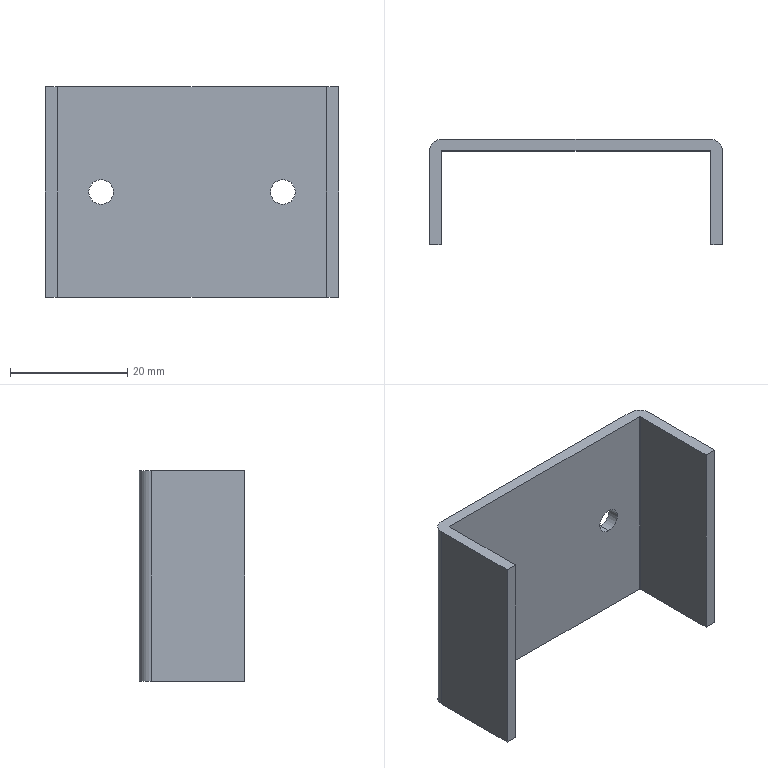Part | STEP file | Closing Plate Clip | 1 solid | 18 faces | box 50 x 18 x 36 mm | volume 5781 mm3 | plane 10 | cylinder 8 | commonest cylinder face diameters 4.2 x6 0.2 x2
STEP:
#1=CARTESIAN_POINT('',(-37.108,9.693,15.9));
#2=VERTEX_POINT('',#1);
#3=CARTESIAN_POINT('',(-37.108,9.693,20.1));
#4=VERTEX_POINT('',#3);
#5=CARTESIAN_POINT('',(-37.108,9.693,18.));
#6=DIRECTION('',(0.,1.,0.));
#7=DIRECTION('',(0.,0.,1.));
#8=AXIS2_PLACEMENT_3D('',#5,#6,#7);
#9=CIRCLE('',#8,2.1);
#10=EDGE_CURVE('',#2,#4,#9,.T.);
#11=ORIENTED_EDGE('',*,*,#10,.F.);
#12=CARTESIAN_POINT('',(-37.108,11.693,15.9));
#13=VERTEX_POINT('',#12);
#14=CARTESIAN_POINT('',(-37.108,1.693,15.9));
#15=DIRECTION('',(0.,1.,0.));
#16=VECTOR('',#15,1000.);
#17=LINE('',#14,#16);
#18=EDGE_CURVE('',#2,#13,#17,.T.);
#19=ORIENTED_EDGE('',*,*,#18,.T.);
#20=CARTESIAN_POINT('',(-37.108,11.693,20.1));
#21=VERTEX_POINT('',#20);
#22=CARTESIAN_POINT('',(-37.108,11.693,18.));
#23=DIRECTION('',(0.,-1.,0.));
#24=DIRECTION('',(0.,0.,1.));
#25=AXIS2_PLACEMENT_3D('',#22,#23,#24);
#26=CIRCLE('',#25,2.1);
#27=EDGE_CURVE('',#21,#13,#26,.T.);
#28=ORIENTED_EDGE('',*,*,#27,.F.);
#29=CARTESIAN_POINT('',(-37.108,1.693,20.1));
#30=DIRECTION('',(0.,1.,0.));
#31=VECTOR('',#30,1000.);
#32=LINE('',#29,#31);
#33=EDGE_CURVE('',#4,#21,#32,.T.);
#34=ORIENTED_EDGE('',*,*,#33,.F.);
#35=EDGE_LOOP('',(#11,#19,#28,#34));
#36=FACE_OUTER_BOUND('',#35,.T.);
#37=CARTESIAN_POINT('',(-37.108,1.693,18.));
#38=DIRECTION('',(0.,1.,0.));
#39=DIRECTION('',(0.,0.,1.));
#40=AXIS2_PLACEMENT_3D('',#37,#38,#39);
#41=CYLINDRICAL_SURFACE('',#40,2.1);
#42=ADVANCED_FACE('',(#36),#41,.F.);
#43=CARTESIAN_POINT('',(-6.108,9.693,15.9));
#44=VERTEX_POINT('',#43);
#45=CARTESIAN_POINT('',(-6.108,9.693,20.1));
#46=VERTEX_POINT('',#45);
#47=CARTESIAN_POINT('',(-6.108,9.693,18.));
#48=DIRECTION('',(0.,1.,0.));
#49=DIRECTION('',(0.,0.,1.));
#50=AXIS2_PLACEMENT_3D('',#47,#48,#49);
#51=CIRCLE('',#50,2.1);
#52=EDGE_CURVE('',#44,#46,#51,.T.);
#53=ORIENTED_EDGE('',*,*,#52,.F.);
#54=CARTESIAN_POINT('',(-6.108,11.693,15.9));
#55=VERTEX_POINT('',#54);
#56=CARTESIAN_POINT('',(-6.108,1.693,15.9));
#57=DIRECTION('',(0.,1.,0.));
#58=VECTOR('',#57,1000.);
#59=LINE('',#56,#58);
#60=EDGE_CURVE('',#44,#55,#59,.T.);
#61=ORIENTED_EDGE('',*,*,#60,.T.);
#62=CARTESIAN_POINT('',(-6.108,11.693,20.1));
#63=VERTEX_POINT('',#62);
#64=CARTESIAN_POINT('',(-6.108,11.693,18.));
#65=DIRECTION('',(0.,-1.,0.));
#66=DIRECTION('',(0.,0.,1.));
#67=AXIS2_PLACEMENT_3D('',#64,#65,#66);
#68=CIRCLE('',#67,2.1);
#69=EDGE_CURVE('',#63,#55,#68,.T.);
#70=ORIENTED_EDGE('',*,*,#69,.F.);
#71=CARTESIAN_POINT('',(-6.108,1.693,20.1));
#72=DIRECTION('',(0.,1.,0.));
#73=VECTOR('',#72,1000.);
#74=LINE('',#71,#73);
#75=EDGE_CURVE('',#46,#63,#74,.T.);
#76=ORIENTED_EDGE('',*,*,#75,.F.);
#77=EDGE_LOOP('',(#53,#61,#70,#76));
#78=FACE_OUTER_BOUND('',#77,.T.);
#79=CARTESIAN_POINT('',(-6.108,1.693,18.));
#80=DIRECTION('',(0.,1.,0.));
#81=DIRECTION('',(0.,0.,1.));
#82=AXIS2_PLACEMENT_3D('',#79,#80,#81);
#83=CYLINDRICAL_SURFACE('',#82,2.1);
#84=ADVANCED_FACE('',(#78),#83,.F.);
#85=CARTESIAN_POINT('',(-44.508,11.693,36.));
#86=VERTEX_POINT('',#85);
#87=CARTESIAN_POINT('',(1.292,11.693,36.));
#88=VERTEX_POINT('',#87);
#89=CARTESIAN_POINT('',(-46.608,11.693,36.));
#90=DIRECTION('',(1.,0.,0.));
#91=VECTOR('',#90,1000.);
#92=LINE('',#89,#91);
#93=EDGE_CURVE('',#86,#88,#92,.T.);
#94=ORIENTED_EDGE('',*,*,#93,.T.);
#95=CARTESIAN_POINT('',(1.292,11.693,0.));
#96=VERTEX_POINT('',#95);
#97=CARTESIAN_POINT('',(1.292,11.693,36.));
#98=DIRECTION('',(0.,0.,-1.));
#99=VECTOR('',#98,1000.);
#100=LINE('',#97,#99);
#101=EDGE_CURVE('',#88,#96,#100,.T.);
#102=ORIENTED_EDGE('',*,*,#101,.T.);
#103=CARTESIAN_POINT('',(-44.508,11.693,0.));
#104=VERTEX_POINT('',#103);
#105=CARTESIAN_POINT('',(-46.608,11.693,0.));
#106=DIRECTION('',(-1.,0.,0.));
#107=VECTOR('',#106,1000.);
#108=LINE('',#105,#107);
#109=EDGE_CURVE('',#96,#104,#108,.T.);
#110=ORIENTED_EDGE('',*,*,#109,.T.);
#111=CARTESIAN_POINT('',(-44.508,11.693,36.));
#112=DIRECTION('',(0.,0.,1.));
#113=VECTOR('',#112,1000.);
#114=LINE('',#111,#113);
#115=EDGE_CURVE('',#104,#86,#114,.T.);
#116=ORIENTED_EDGE('',*,*,#115,.T.);
#117=EDGE_LOOP('',(#94,#102,#110,#116));
#118=FACE_OUTER_BOUND('',#117,.T.);
#119=ORIENTED_EDGE('',*,*,#27,.T.);
#120=CARTESIAN_POINT('',(-37.108,11.693,18.));
#121=DIRECTION('',(0.,-1.,0.));
#122=DIRECTION('',(0.,0.,1.));
#123=AXIS2_PLACEMENT_3D('',#120,#121,#122);
#124=CIRCLE('',#123,2.1);
#125=EDGE_CURVE('',#13,#21,#124,.T.);
#126=ORIENTED_EDGE('',*,*,#125,.T.);
#127=EDGE_LOOP('',(#119,#126));
#128=FACE_BOUND('',#127,.T.);
#129=ORIENTED_EDGE('',*,*,#69,.T.);
#130=CARTESIAN_POINT('',(-6.108,11.693,18.));
#131=DIRECTION('',(0.,-1.,0.));
#132=DIRECTION('',(0.,0.,1.));
#133=AXIS2_PLACEMENT_3D('',#130,#131,#132);
#134=CIRCLE('',#133,2.1);
#135=EDGE_CURVE('',#55,#63,#134,.T.);
#136=ORIENTED_EDGE('',*,*,#135,.T.);
#137=EDGE_LOOP('',(#129,#136));
#138=FACE_BOUND('',#137,.T.);
#139=CARTESIAN_POINT('',(-46.608,11.693,36.));
#140=DIRECTION('',(0.,1.,0.));
#141=DIRECTION('',(0.,0.,1.));
#142=AXIS2_PLACEMENT_3D('',#139,#140,#141);
#143=PLANE('',#142);
#144=ADVANCED_FACE('',(#118,#128,#138),#143,.T.);
#145=CARTESIAN_POINT('',(3.392,9.593,36.));
#146=VERTEX_POINT('',#145);
#147=CARTESIAN_POINT('',(1.292,9.593,36.));
#148=DIRECTION('',(0.,0.,-1.));
#149=DIRECTION('',(-1.,0.,0.));
#150=AXIS2_PLACEMENT_3D('',#147,#148,#149);
#151=CIRCLE('',#150,2.1);
#152=EDGE_CURVE('',#88,#146,#151,.T.);
#153=ORIENTED_EDGE('',*,*,#152,.T.);
#154=CARTESIAN_POINT('',(3.392,9.593,0.));
#155=VERTEX_POINT('',#154);
#156=CARTESIAN_POINT('',(3.392,9.593,36.));
#157=DIRECTION('',(0.,0.,-1.));
#158=VECTOR('',#157,1000.);
#159=LINE('',#156,#158);
#160=EDGE_CURVE('',#146,#155,#159,.T.);
#161=ORIENTED_EDGE('',*,*,#160,.T.);
#162=CARTESIAN_POINT('',(1.292,9.593,0.));
#163=DIRECTION('',(0.,0.,1.));
#164=DIRECTION('',(-1.,0.,0.));
#165=AXIS2_PLACEMENT_3D('',#162,#163,#164);
#166=CIRCLE('',#165,2.1);
#167=EDGE_CURVE('',#155,#96,#166,.T.);
#168=ORIENTED_EDGE('',*,*,#167,.T.);
#169=ORIENTED_EDGE('',*,*,#101,.F.);
#170=EDGE_LOOP('',(#153,#161,#168,#169));
#171=FACE_OUTER_BOUND('',#170,.T.);
#172=CARTESIAN_POINT('',(1.292,9.593,36.));
#173=DIRECTION('',(0.,0.,-1.));
#174=DIRECTION('',(-1.,0.,0.));
#175=AXIS2_PLACEMENT_3D('',#172,#173,#174);
#176=CYLINDRICAL_SURFACE('',#175,2.1);
#177=ADVANCED_FACE('',(#171),#176,.T.);
#178=CARTESIAN_POINT('',(-44.508,9.693,36.));
#179=VERTEX_POINT('',#178);
#180=CARTESIAN_POINT('',(1.292,9.693,36.));
#181=VERTEX_POINT('',#180);
#182=CARTESIAN_POINT('',(-44.608,9.693,36.));
#183=DIRECTION('',(1.,0.,0.));
#184=VECTOR('',#183,1000.);
#185=LINE('',#182,#184);
#186=EDGE_CURVE('',#179,#181,#185,.T.);
#187=ORIENTED_EDGE('',*,*,#186,.T.);
#188=CARTESIAN_POINT('',(1.392,9.593,36.));
#189=VERTEX_POINT('',#188);
#190=CARTESIAN_POINT('',(1.292,9.593,36.));
#191=DIRECTION('',(0.,0.,-1.));
#192=DIRECTION('',(-1.,0.,0.));
#193=AXIS2_PLACEMENT_3D('',#190,#191,#192);
#194=CIRCLE('',#193,0.1);
#195=EDGE_CURVE('',#181,#189,#194,.T.);
#196=ORIENTED_EDGE('',*,*,#195,.T.);
#197=CARTESIAN_POINT('',(1.392,-6.307,36.));
#198=VERTEX_POINT('',#197);
#199=CARTESIAN_POINT('',(1.392,9.693,36.));
#200=DIRECTION('',(0.,-1.,0.));
#201=VECTOR('',#200,1000.);
#202=LINE('',#199,#201);
#203=EDGE_CURVE('',#189,#198,#202,.T.);
#204=ORIENTED_EDGE('',*,*,#203,.T.);
#205=CARTESIAN_POINT('',(3.392,-6.307,36.));
#206=VERTEX_POINT('',#205);
#207=CARTESIAN_POINT('',(3.392,-6.307,36.));
#208=DIRECTION('',(-1.,0.,0.));
#209=VECTOR('',#208,1000.);
#210=LINE('',#207,#209);
#211=EDGE_CURVE('',#206,#198,#210,.T.);
#212=ORIENTED_EDGE('',*,*,#211,.F.);
#213=CARTESIAN_POINT('',(3.392,11.693,36.));
#214=DIRECTION('',(0.,-1.,0.));
#215=VECTOR('',#214,1000.);
#216=LINE('',#213,#215);
#217=EDGE_CURVE('',#146,#206,#216,.T.);
#218=ORIENTED_EDGE('',*,*,#217,.F.);
#219=ORIENTED_EDGE('',*,*,#152,.F.);
#220=ORIENTED_EDGE('',*,*,#93,.F.);
#221=CARTESIAN_POINT('',(-46.608,9.593,36.));
#222=VERTEX_POINT('',#221);
#223=CARTESIAN_POINT('',(-44.508,9.593,36.));
#224=DIRECTION('',(0.,0.,-1.));
#225=DIRECTION('',(-1.,0.,0.));
#226=AXIS2_PLACEMENT_3D('',#223,#224,#225);
#227=CIRCLE('',#226,2.1);
#228=EDGE_CURVE('',#222,#86,#227,.T.);
#229=ORIENTED_EDGE('',*,*,#228,.F.);
#230=CARTESIAN_POINT('',(-46.608,-6.307,36.));
#231=VERTEX_POINT('',#230);
#232=CARTESIAN_POINT('',(-46.608,-6.307,36.));
#233=DIRECTION('',(0.,1.,0.));
#234=VECTOR('',#233,1000.);
#235=LINE('',#232,#234);
#236=EDGE_CURVE('',#231,#222,#235,.T.);
#237=ORIENTED_EDGE('',*,*,#236,.F.);
#238=CARTESIAN_POINT('',(-44.608,-6.307,36.));
#239=VERTEX_POINT('',#238);
#240=CARTESIAN_POINT('',(1.292,-6.307,36.));
#241=DIRECTION('',(1.,0.,0.));
#242=VECTOR('',#241,1000.);
#243=LINE('',#240,#242);
#244=EDGE_CURVE('',#231,#239,#243,.T.);
#245=ORIENTED_EDGE('',*,*,#244,.T.);
#246=CARTESIAN_POINT('',(-44.608,9.593,36.));
#247=VERTEX_POINT('',#246);
#248=CARTESIAN_POINT('',(-44.608,9.593,36.));
#249=DIRECTION('',(0.,1.,0.));
#250=VECTOR('',#249,1000.);
#251=LINE('',#248,#250);
#252=EDGE_CURVE('',#239,#247,#251,.T.);
#253=ORIENTED_EDGE('',*,*,#252,.T.);
#254=CARTESIAN_POINT('',(-44.508,9.593,36.));
#255=DIRECTION('',(0.,0.,-1.));
#256=DIRECTION('',(-1.,0.,0.));
#257=AXIS2_PLACEMENT_3D('',#254,#255,#256);
#258=CIRCLE('',#257,0.1);
#259=EDGE_CURVE('',#247,#179,#258,.T.);
#260=ORIENTED_EDGE('',*,*,#259,.T.);
#261=EDGE_LOOP('',(#187,#196,#204,#212,#218,#219,#220,#229,#237,#245,#253,#260));
#262=FACE_OUTER_BOUND('',#261,.T.);
#263=CARTESIAN_POINT('',(-44.608,9.593,36.));
#264=DIRECTION('',(0.,0.,1.));
#265=DIRECTION('',(1.,0.,0.));
#266=AXIS2_PLACEMENT_3D('',#263,#264,#265);
#267=PLANE('',#266);
#268=ADVANCED_FACE('',(#262),#267,.T.);
#269=ORIENTED_EDGE('',*,*,#228,.T.);
#270=ORIENTED_EDGE('',*,*,#115,.F.);
#271=CARTESIAN_POINT('',(-46.608,9.593,0.));
#272=VERTEX_POINT('',#271);
#273=CARTESIAN_POINT('',(-44.508,9.593,0.));
#274=DIRECTION('',(0.,0.,1.));
#275=DIRECTION('',(-1.,0.,0.));
#276=AXIS2_PLACEMENT_3D('',#273,#274,#275);
#277=CIRCLE('',#276,2.1);
#278=EDGE_CURVE('',#104,#272,#277,.T.);
#279=ORIENTED_EDGE('',*,*,#278,.T.);
#280=CARTESIAN_POINT('',(-46.608,9.593,36.));
#281=DIRECTION('',(0.,0.,1.));
#282=VECTOR('',#281,1000.);
#283=LINE('',#280,#282);
#284=EDGE_CURVE('',#272,#222,#283,.T.);
#285=ORIENTED_EDGE('',*,*,#284,.T.);
#286=EDGE_LOOP('',(#269,#270,#279,#285));
#287=FACE_OUTER_BOUND('',#286,.T.);
#288=CARTESIAN_POINT('',(-44.508,9.593,36.));
#289=DIRECTION('',(0.,0.,-1.));
#290=DIRECTION('',(-1.,0.,0.));
#291=AXIS2_PLACEMENT_3D('',#288,#289,#290);
#292=CYLINDRICAL_SURFACE('',#291,2.1);
#293=ADVANCED_FACE('',(#287),#292,.T.);
#294=CARTESIAN_POINT('',(1.292,9.693,0.));
#295=VERTEX_POINT('',#294);
#296=CARTESIAN_POINT('',(-44.508,9.693,0.));
#297=VERTEX_POINT('',#296);
#298=CARTESIAN_POINT('',(1.392,9.693,0.));
#299=DIRECTION('',(-1.,0.,0.));
#300=VECTOR('',#299,1000.);
#301=LINE('',#298,#300);
#302=EDGE_CURVE('',#295,#297,#301,.T.);
#303=ORIENTED_EDGE('',*,*,#302,.T.);
#304=CARTESIAN_POINT('',(-44.608,9.593,0.));
#305=VERTEX_POINT('',#304);
#306=CARTESIAN_POINT('',(-44.508,9.593,0.));
#307=DIRECTION('',(0.,0.,1.));
#308=DIRECTION('',(-1.,0.,0.));
#309=AXIS2_PLACEMENT_3D('',#306,#307,#308);
#310=CIRCLE('',#309,0.1);
#311=EDGE_CURVE('',#297,#305,#310,.T.);
#312=ORIENTED_EDGE('',*,*,#311,.T.);
#313=CARTESIAN_POINT('',(-44.608,-6.307,0.));
#314=VERTEX_POINT('',#313);
#315=CARTESIAN_POINT('',(-44.608,9.693,0.));
#316=DIRECTION('',(0.,-1.,0.));
#317=VECTOR('',#316,1000.);
#318=LINE('',#315,#317);
#319=EDGE_CURVE('',#305,#314,#318,.T.);
#320=ORIENTED_EDGE('',*,*,#319,.T.);
#321=CARTESIAN_POINT('',(-46.608,-6.307,0.));
#322=VERTEX_POINT('',#321);
#323=CARTESIAN_POINT('',(-44.608,-6.307,0.));
#324=DIRECTION('',(1.,0.,0.));
#325=VECTOR('',#324,1000.);
#326=LINE('',#323,#325);
#327=EDGE_CURVE('',#322,#314,#326,.T.);
#328=ORIENTED_EDGE('',*,*,#327,.F.);
#329=CARTESIAN_POINT('',(-46.608,-6.307,0.));
#330=DIRECTION('',(0.,-1.,0.));
#331=VECTOR('',#330,1000.);
#332=LINE('',#329,#331);
#333=EDGE_CURVE('',#272,#322,#332,.T.);
#334=ORIENTED_EDGE('',*,*,#333,.F.);
#335=ORIENTED_EDGE('',*,*,#278,.F.);
#336=ORIENTED_EDGE('',*,*,#109,.F.);
#337=ORIENTED_EDGE('',*,*,#167,.F.);
#338=CARTESIAN_POINT('',(3.392,-6.307,0.));
#339=VERTEX_POINT('',#338);
#340=CARTESIAN_POINT('',(3.392,11.693,0.));
#341=DIRECTION('',(0.,1.,0.));
#342=VECTOR('',#341,1000.);
#343=LINE('',#340,#342);
#344=EDGE_CURVE('',#339,#155,#343,.T.);
#345=ORIENTED_EDGE('',*,*,#344,.F.);
#346=CARTESIAN_POINT('',(1.392,-6.307,0.));
#347=VERTEX_POINT('',#346);
#348=CARTESIAN_POINT('',(3.392,-6.307,0.));
#349=DIRECTION('',(1.,0.,0.));
#350=VECTOR('',#349,1000.);
#351=LINE('',#348,#350);
#352=EDGE_CURVE('',#347,#339,#351,.T.);
#353=ORIENTED_EDGE('',*,*,#352,.F.);
#354=CARTESIAN_POINT('',(1.392,9.593,0.));
#355=VERTEX_POINT('',#354);
#356=CARTESIAN_POINT('',(1.392,9.593,0.));
#357=DIRECTION('',(0.,-1.,0.));
#358=VECTOR('',#357,1000.);
#359=LINE('',#356,#358);
#360=EDGE_CURVE('',#355,#347,#359,.T.);
#361=ORIENTED_EDGE('',*,*,#360,.F.);
#362=CARTESIAN_POINT('',(1.292,9.593,0.));
#363=DIRECTION('',(0.,0.,1.));
#364=DIRECTION('',(-1.,0.,0.));
#365=AXIS2_PLACEMENT_3D('',#362,#363,#364);
#366=CIRCLE('',#365,0.1);
#367=EDGE_CURVE('',#355,#295,#366,.T.);
#368=ORIENTED_EDGE('',*,*,#367,.T.);
#369=EDGE_LOOP('',(#303,#312,#320,#328,#334,#335,#336,#337,#345,#353,#361,#368));
#370=FACE_OUTER_BOUND('',#369,.T.);
#371=CARTESIAN_POINT('',(1.392,9.593,0.));
#372=DIRECTION('',(0.,0.,-1.));
#373=DIRECTION('',(-1.,0.,0.));
#374=AXIS2_PLACEMENT_3D('',#371,#372,#373);
#375=PLANE('',#374);
#376=ADVANCED_FACE('',(#370),#375,.T.);
#377=ORIENTED_EDGE('',*,*,#18,.F.);
#378=CARTESIAN_POINT('',(-37.108,9.693,18.));
#379=DIRECTION('',(0.,1.,0.));
#380=DIRECTION('',(0.,0.,1.));
#381=AXIS2_PLACEMENT_3D('',#378,#379,#380);
#382=CIRCLE('',#381,2.1);
#383=EDGE_CURVE('',#4,#2,#382,.T.);
#384=ORIENTED_EDGE('',*,*,#383,.F.);
#385=ORIENTED_EDGE('',*,*,#33,.T.);
#386=ORIENTED_EDGE('',*,*,#125,.F.);
#387=EDGE_LOOP('',(#377,#384,#385,#386));
#388=FACE_OUTER_BOUND('',#387,.T.);
#389=CARTESIAN_POINT('',(-37.108,1.693,18.));
#390=DIRECTION('',(0.,1.,0.));
#391=DIRECTION('',(0.,0.,1.));
#392=AXIS2_PLACEMENT_3D('',#389,#390,#391);
#393=CYLINDRICAL_SURFACE('',#392,2.1);
#394=ADVANCED_FACE('',(#388),#393,.F.);
#395=ORIENTED_EDGE('',*,*,#60,.F.);
#396=CARTESIAN_POINT('',(-6.108,9.693,18.));
#397=DIRECTION('',(0.,1.,0.));
#398=DIRECTION('',(0.,0.,1.));
#399=AXIS2_PLACEMENT_3D('',#396,#397,#398);
#400=CIRCLE('',#399,2.1);
#401=EDGE_CURVE('',#46,#44,#400,.T.);
#402=ORIENTED_EDGE('',*,*,#401,.F.);
#403=ORIENTED_EDGE('',*,*,#75,.T.);
#404=ORIENTED_EDGE('',*,*,#135,.F.);
#405=EDGE_LOOP('',(#395,#402,#403,#404));
#406=FACE_OUTER_BOUND('',#405,.T.);
#407=CARTESIAN_POINT('',(-6.108,1.693,18.));
#408=DIRECTION('',(0.,1.,0.));
#409=DIRECTION('',(0.,0.,1.));
#410=AXIS2_PLACEMENT_3D('',#407,#408,#409);
#411=CYLINDRICAL_SURFACE('',#410,2.1);
#412=ADVANCED_FACE('',(#406),#411,.F.);
#413=ORIENTED_EDGE('',*,*,#217,.T.);
#414=CARTESIAN_POINT('',(3.392,-6.307,36.));
#415=DIRECTION('',(0.,0.,-1.));
#416=VECTOR('',#415,1000.);
#417=LINE('',#414,#416);
#418=EDGE_CURVE('',#206,#339,#417,.T.);
#419=ORIENTED_EDGE('',*,*,#418,.T.);
#420=ORIENTED_EDGE('',*,*,#344,.T.);
#421=ORIENTED_EDGE('',*,*,#160,.F.);
#422=EDGE_LOOP('',(#413,#419,#420,#421));
#423=FACE_OUTER_BOUND('',#422,.T.);
#424=CARTESIAN_POINT('',(3.392,11.693,36.));
#425=DIRECTION('',(1.,0.,0.));
#426=DIRECTION('',(0.,1.,0.));
#427=AXIS2_PLACEMENT_3D('',#424,#425,#426);
#428=PLANE('',#427);
#429=ADVANCED_FACE('',(#423),#428,.T.);
#430=CARTESIAN_POINT('',(1.292,9.693,36.));
#431=DIRECTION('',(0.,0.,-1.));
#432=VECTOR('',#431,1000.);
#433=LINE('',#430,#432);
#434=EDGE_CURVE('',#181,#295,#433,.T.);
#435=ORIENTED_EDGE('',*,*,#434,.F.);
#436=ORIENTED_EDGE('',*,*,#186,.F.);
#437=CARTESIAN_POINT('',(-44.508,9.693,36.));
#438=DIRECTION('',(0.,0.,1.));
#439=VECTOR('',#438,1000.);
#440=LINE('',#437,#439);
#441=EDGE_CURVE('',#297,#179,#440,.T.);
#442=ORIENTED_EDGE('',*,*,#441,.F.);
#443=ORIENTED_EDGE('',*,*,#302,.F.);
#444=EDGE_LOOP('',(#435,#436,#442,#443));
#445=FACE_OUTER_BOUND('',#444,.T.);
#446=ORIENTED_EDGE('',*,*,#383,.T.);
#447=ORIENTED_EDGE('',*,*,#10,.T.);
#448=EDGE_LOOP('',(#446,#447));
#449=FACE_BOUND('',#448,.T.);
#450=ORIENTED_EDGE('',*,*,#401,.T.);
#451=ORIENTED_EDGE('',*,*,#52,.T.);
#452=EDGE_LOOP('',(#450,#451));
#453=FACE_BOUND('',#452,.T.);
#454=CARTESIAN_POINT('',(-46.608,9.693,36.));
#455=DIRECTION('',(0.,1.,0.));
#456=DIRECTION('',(0.,0.,1.));
#457=AXIS2_PLACEMENT_3D('',#454,#455,#456);
#458=PLANE('',#457);
#459=ADVANCED_FACE('',(#445,#449,#453),#458,.F.);
#460=ORIENTED_EDGE('',*,*,#236,.T.);
#461=ORIENTED_EDGE('',*,*,#284,.F.);
#462=ORIENTED_EDGE('',*,*,#333,.T.);
#463=CARTESIAN_POINT('',(-46.608,-6.307,36.));
#464=DIRECTION('',(0.,0.,1.));
#465=VECTOR('',#464,1000.);
#466=LINE('',#463,#465);
#467=EDGE_CURVE('',#322,#231,#466,.T.);
#468=ORIENTED_EDGE('',*,*,#467,.T.);
#469=EDGE_LOOP('',(#460,#461,#462,#468));
#470=FACE_OUTER_BOUND('',#469,.T.);
#471=CARTESIAN_POINT('',(-46.608,-6.307,36.));
#472=DIRECTION('',(-1.,0.,0.));
#473=DIRECTION('',(0.,0.,1.));
#474=AXIS2_PLACEMENT_3D('',#471,#472,#473);
#475=PLANE('',#474);
#476=ADVANCED_FACE('',(#470),#475,.T.);
#477=ORIENTED_EDGE('',*,*,#211,.T.);
#478=CARTESIAN_POINT('',(1.392,-6.307,36.));
#479=DIRECTION('',(0.,0.,-1.));
#480=VECTOR('',#479,1000.);
#481=LINE('',#478,#480);
#482=EDGE_CURVE('',#198,#347,#481,.T.);
#483=ORIENTED_EDGE('',*,*,#482,.T.);
#484=ORIENTED_EDGE('',*,*,#352,.T.);
#485=ORIENTED_EDGE('',*,*,#418,.F.);
#486=EDGE_LOOP('',(#477,#483,#484,#485));
#487=FACE_OUTER_BOUND('',#486,.T.);
#488=CARTESIAN_POINT('',(3.392,-6.307,36.));
#489=DIRECTION('',(0.,-1.,0.));
#490=DIRECTION('',(0.,0.,-1.));
#491=AXIS2_PLACEMENT_3D('',#488,#489,#490);
#492=PLANE('',#491);
#493=ADVANCED_FACE('',(#487),#492,.T.);
#494=CARTESIAN_POINT('',(1.392,9.593,36.));
#495=DIRECTION('',(0.,0.,-1.));
#496=VECTOR('',#495,1000.);
#497=LINE('',#494,#496);
#498=EDGE_CURVE('',#189,#355,#497,.T.);
#499=ORIENTED_EDGE('',*,*,#498,.F.);
#500=ORIENTED_EDGE('',*,*,#195,.F.);
#501=ORIENTED_EDGE('',*,*,#434,.T.);
#502=ORIENTED_EDGE('',*,*,#367,.F.);
#503=EDGE_LOOP('',(#499,#500,#501,#502));
#504=FACE_OUTER_BOUND('',#503,.T.);
#505=CARTESIAN_POINT('',(1.292,9.593,36.));
#506=DIRECTION('',(0.,0.,-1.));
#507=DIRECTION('',(-1.,0.,0.));
#508=AXIS2_PLACEMENT_3D('',#505,#506,#507);
#509=CYLINDRICAL_SURFACE('',#508,0.1);
#510=ADVANCED_FACE('',(#504),#509,.F.);
#511=ORIENTED_EDGE('',*,*,#441,.T.);
#512=ORIENTED_EDGE('',*,*,#259,.F.);
#513=CARTESIAN_POINT('',(-44.608,9.593,36.));
#514=DIRECTION('',(0.,0.,1.));
#515=VECTOR('',#514,1000.);
#516=LINE('',#513,#515);
#517=EDGE_CURVE('',#305,#247,#516,.T.);
#518=ORIENTED_EDGE('',*,*,#517,.F.);
#519=ORIENTED_EDGE('',*,*,#311,.F.);
#520=EDGE_LOOP('',(#511,#512,#518,#519));
#521=FACE_OUTER_BOUND('',#520,.T.);
#522=CARTESIAN_POINT('',(-44.508,9.593,36.));
#523=DIRECTION('',(0.,0.,-1.));
#524=DIRECTION('',(-1.,0.,0.));
#525=AXIS2_PLACEMENT_3D('',#522,#523,#524);
#526=CYLINDRICAL_SURFACE('',#525,0.1);
#527=ADVANCED_FACE('',(#521),#526,.F.);
#528=ORIENTED_EDGE('',*,*,#244,.F.);
#529=ORIENTED_EDGE('',*,*,#467,.F.);
#530=ORIENTED_EDGE('',*,*,#327,.T.);
#531=CARTESIAN_POINT('',(-44.608,-6.307,36.));
#532=DIRECTION('',(0.,0.,1.));
#533=VECTOR('',#532,1000.);
#534=LINE('',#531,#533);
#535=EDGE_CURVE('',#314,#239,#534,.T.);
#536=ORIENTED_EDGE('',*,*,#535,.T.);
#537=EDGE_LOOP('',(#528,#529,#530,#536));
#538=FACE_OUTER_BOUND('',#537,.T.);
#539=CARTESIAN_POINT('',(-44.608,-6.307,36.));
#540=DIRECTION('',(0.,-1.,0.));
#541=DIRECTION('',(0.,0.,-1.));
#542=AXIS2_PLACEMENT_3D('',#539,#540,#541);
#543=PLANE('',#542);
#544=ADVANCED_FACE('',(#538),#543,.T.);
#545=ORIENTED_EDGE('',*,*,#482,.F.);
#546=ORIENTED_EDGE('',*,*,#203,.F.);
#547=ORIENTED_EDGE('',*,*,#498,.T.);
#548=ORIENTED_EDGE('',*,*,#360,.T.);
#549=EDGE_LOOP('',(#545,#546,#547,#548));
#550=FACE_OUTER_BOUND('',#549,.T.);
#551=CARTESIAN_POINT('',(1.392,11.693,36.));
#552=DIRECTION('',(1.,0.,0.));
#553=DIRECTION('',(0.,1.,0.));
#554=AXIS2_PLACEMENT_3D('',#551,#552,#553);
#555=PLANE('',#554);
#556=ADVANCED_FACE('',(#550),#555,.F.);
#557=ORIENTED_EDGE('',*,*,#517,.T.);
#558=ORIENTED_EDGE('',*,*,#252,.F.);
#559=ORIENTED_EDGE('',*,*,#535,.F.);
#560=ORIENTED_EDGE('',*,*,#319,.F.);
#561=EDGE_LOOP('',(#557,#558,#559,#560));
#562=FACE_OUTER_BOUND('',#561,.T.);
#563=CARTESIAN_POINT('',(-44.608,-6.307,36.));
#564=DIRECTION('',(-1.,0.,0.));
#565=DIRECTION('',(0.,0.,1.));
#566=AXIS2_PLACEMENT_3D('',#563,#564,#565);
#567=PLANE('',#566);
#568=ADVANCED_FACE('',(#562),#567,.F.);
#569=CLOSED_SHELL('',(#42,#84,#144,#177,#268,#293,#376,#394,#412,#429,#459,#476,#493,#510,#527,#544,#556,#568));
#570=MANIFOLD_SOLID_BREP('',#569);
#571=CARTESIAN_POINT('',(0.,0.,0.));
#572=DIRECTION('',(0.,0.,1.));
#573=DIRECTION('',(1.,0.,0.));
#574=AXIS2_PLACEMENT_3D('',#571,#572,#573);
#575=(LENGTH_UNIT()NAMED_UNIT(*)SI_UNIT(.MILLI.,.METRE.));
#576=UNCERTAINTY_MEASURE_WITH_UNIT(LENGTH_MEASURE(0.00001),#575,'','');
#577=(NAMED_UNIT(*)PLANE_ANGLE_UNIT()SI_UNIT($,.RADIAN.));
#578=(NAMED_UNIT(*)SI_UNIT($,.STERADIAN.)SOLID_ANGLE_UNIT());
#579=(GEOMETRIC_REPRESENTATION_CONTEXT(3)GLOBAL_UNCERTAINTY_ASSIGNED_CONTEXT((#576))GLOBAL_UNIT_ASSIGNED_CONTEXT((#575,#577,#578))REPRESENTATION_CONTEXT('',''));
#580=ADVANCED_BREP_SHAPE_REPRESENTATION('',(#570,#574),#579);